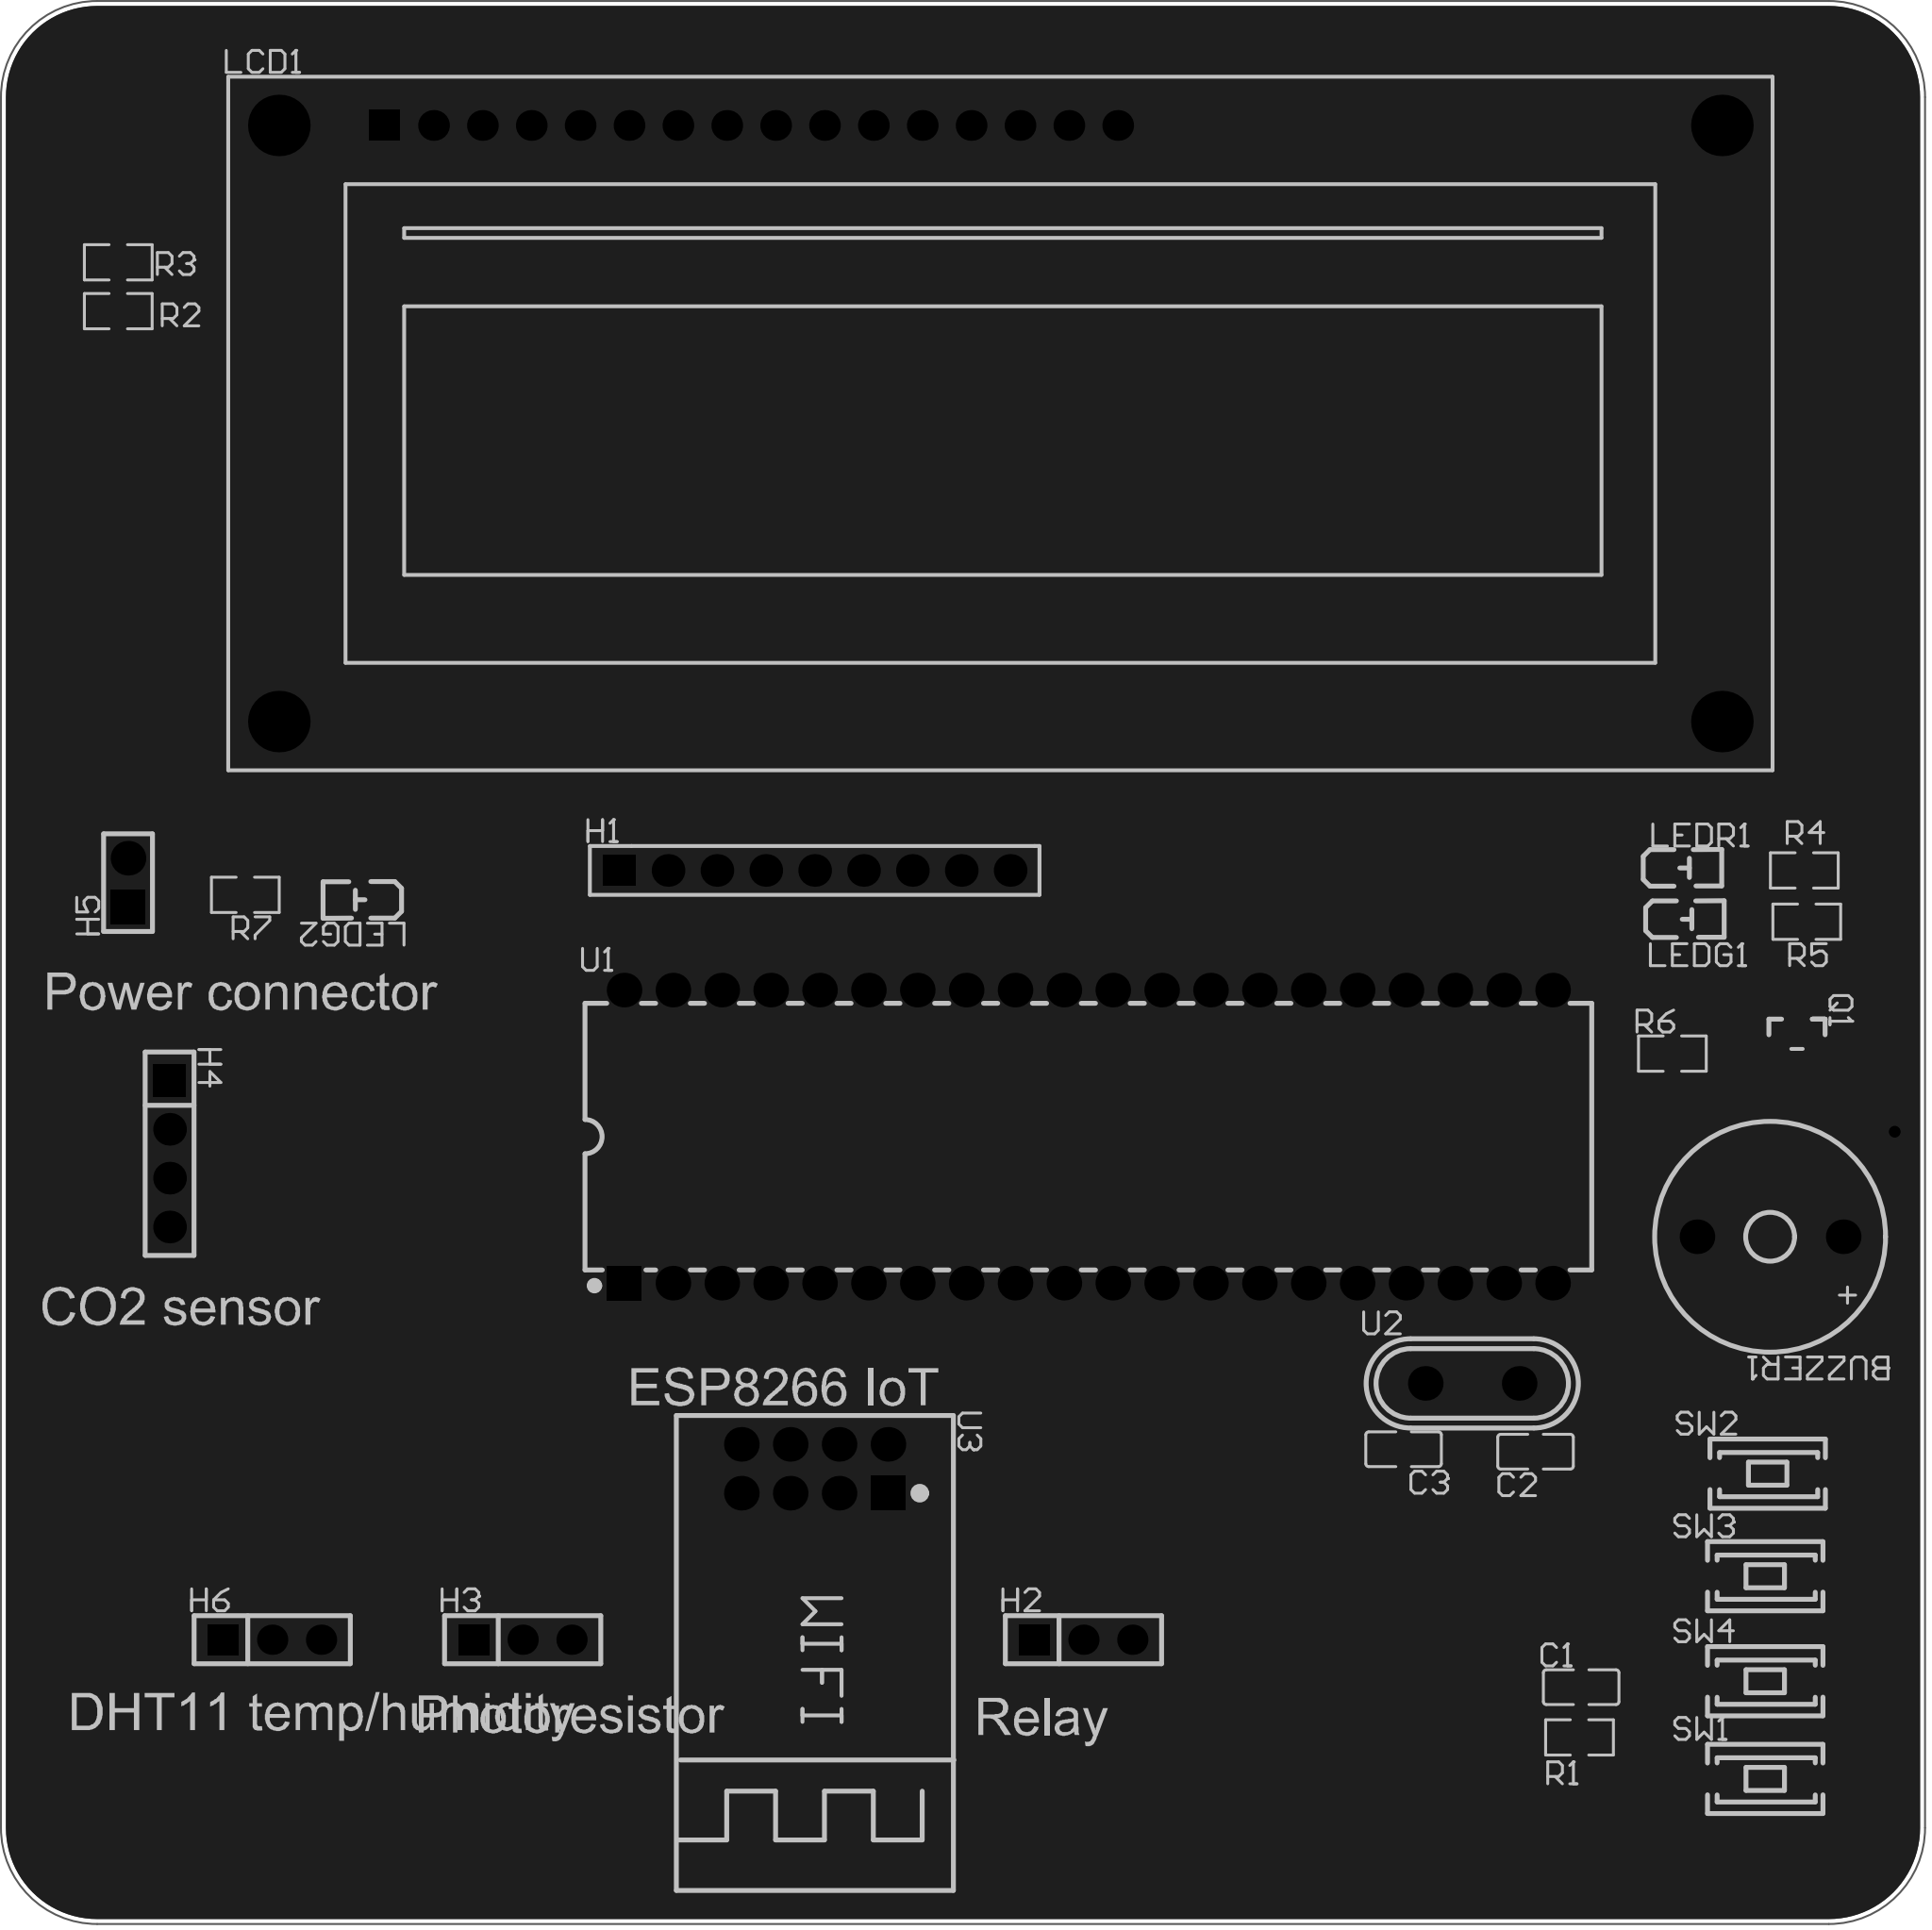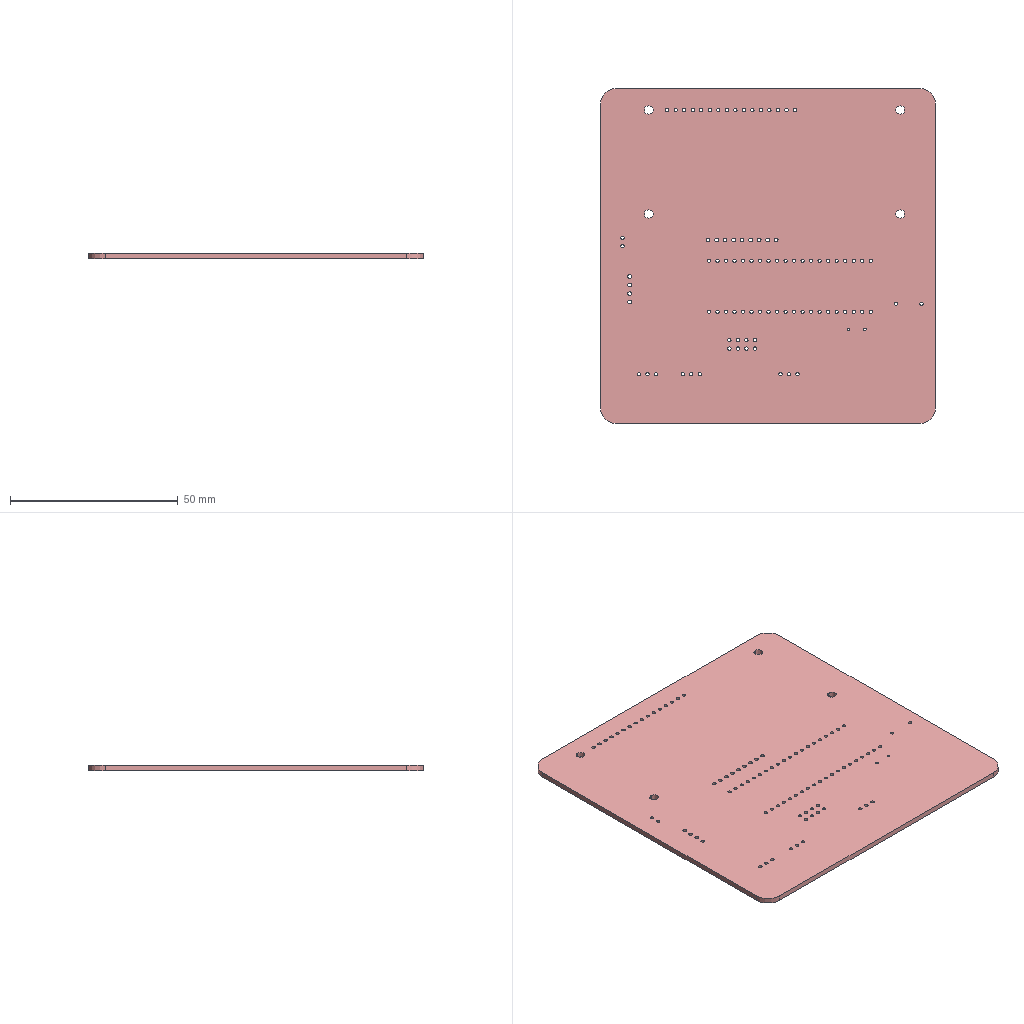Circuit board layout | Altium Designer | box 100 x 100 x 1.6 mm
Layer stack:
# Altium Designer layer stack of  (unit mm; dielectric type: 0 none, 1 core, 2 prepreg, 3 surface material)
index,name,kind,layer,copper_thickness_mm,dielectric_type,dielectric_thickness_mm,dielectric_material,dielectric_constant
0,Top Paste Mask Layer,other,,,,,,
1,Top Silkscreen Layer,other,,,,,,
2,Top Solder Mask Layer,dielectric,,,3,0.01,,3.3
3,Top Layer,copper,Top Layer,0.035,,,,
4,Dielectric1,dielectric,,,3,1.51,FR4,4.5
5,Bottom Layer,copper,Bottom Layer,0.035,,,,
6,Bottom Solder Mask Layer,dielectric,,,3,0.01,,3.3
7,Bottom Silkscreen Layer,other,,,,,,
8,Bottom Paste Mask Layer,other,,,,,,
# drill layer pairs: low layer,high layer
drill_pair,Top Layer,Bottom Layer
Part placement:
Designator,Comment,Layer,Footprint,Center-X(mm),Center-Y(mm),Rotation
BUZZER1,buzzer-12X9,TopLayer,BUZ-TH_BD12.0-P7.60-D0.6-FD,175.768,117.475,180
C1,10uf,TopLayer,C0805,165.947,94.052,0
C2,30pf,TopLayer,C0805,156.718,106.426,0
C3,30pf,TopLayer,C0805,163.576,106.299,180
H1,,TopLayer,HDR-TH_9P-P2.54-V-F-1,126.111,136.525,0
LCD1,LMB162ADC,TopLayer,LCD1602,135.763,159.766,0
LEDG1,,TopLayer,LED_0805,171.4,133.99,0
LEDR1,,TopLayer,LED_0805,171.273,136.657,0
Q1,2N3906S-RTK/PS,TopLayer,SOT-23-3_L2.9-W1.3-P1.90-LS2.4-TR,177.165,128.143,270
R1,10K,TopLayer,R0805,165.862,91.44,0
R2,10K,TopLayer,R0805,89.916,165.608,180
R3,1K,TopLayer,R0805,89.916,168.148,0
R4,220,TopLayer,R0805,177.546,136.525,0
R5,220,TopLayer,R0805,177.673,133.858,0
R6,2.2K,TopLayer,R0805,170.688,127,0
U1,STC89C516RD+40I-PDIP40,TopLayer,DIP-40_L52.3-W13.9-P2.54-LS15.2-BL,140.335,122.682,0
U2,11.059MHz,TopLayer,HC-49US_L11.0-W4.6-P4.88,160.287,109.85,0
LEDG2,,TopLayer,LED_0805,102.539,134.996,180
R7,220,TopLayer,R0805,96.52,135.255,180
H5,,TopLayer,HDR-TH_2P-P2.54-V-M-1,90.424,135.89,90
SW1,Tact switch 3*6*2.5,TopLayer,SW-SMD_L6.0-W3.6-LS8.0,175.514,89.281,0
SW2,Tact switch 3*6*2.5,TopLayer,SW-SMD_L6.0-W3.6-LS8.0,175.641,105.156,0
SW3,Tact switch 3*6*2.5,TopLayer,SW-SMD_L6.0-W3.6-LS8.0,175.514,99.822,0
SW4,Tact switch 3*6*2.5,TopLayer,SW-SMD_L6.0-W3.6-LS8.0,175.514,94.361,0
H2,,TopLayer,HDR-TH_3P-P2.54-V-F,140.081,96.52,0
H3,,TopLayer,HDR-TH_3P-P2.54-V-F,110.934,96.52,0
H4,,TopLayer,HDR-TH_4P-P2.54-V-F,92.583,121.793,270
H6,,TopLayer,HDR-TH_3P-P2.54-V-F,97.917,96.52,0
U3,Ai-Thinker ESP-01S ESP8266,TopLayer,WIFIM-TH_8P-L24.7-W14.4-P2.54,126.111,105.41,270
Pad and via stacks:
# Altium Designer via and pad stacks of  (unit mm). Each distinct definition once, with the count of objects using it.
# via: kind,start_layer,end_layer,hole_mm,diameter_mm,mode(0 simple;1 top-mid-bottom;2 full stack),diameter_per_layer,count,example_net
# pad: kind,layer,hole_mm,hole_type(0 round;1 square;2 slot),plating,top_size,top_shape(1 round;2 rect;3 octagon;9 rounded rect),mid_size,bottom_size,mode,footprint,size_per_layer,count,example
pad,Multi-Layer,1,0,plated,1.8x1.8,1,1.8x1.8,1.8x1.8,0,BUZ-TH_BD12.0-P7.60-D0.6-FD,,2,BUZZER1.2
pad,Multi-Layer,1.1,0,plated,1.7x1.575,2,1.7x1.575,1.7x1.575,0,HDR-TH_9P-P2.54-V-F-1,,1,H1.1
pad,Multi-Layer,1.1,0,plated,1.7x1.7,1,1.7x1.7,1.7x1.7,0,HDR-TH_9P-P2.54-V-F-1,,8,H1.2
pad,Multi-Layer,1,0,plated,1.6x1.6,1,1.6x1.6,1.6x1.6,0,LCD1602,,15,LCD1.16
pad,Multi-Layer,1,0,plated,1.6x1.6,2,1.6x1.6,1.6x1.6,0,LCD1602,,1,LCD1.1
pad,Multi-Layer,2.5,2,plated,3.2x3.2,1,3.2x3.2,3.2x3.2,0,LCD1602,,4,LCD1.0
pad,Multi-Layer,1,0,plated,1.8x1.8,1,1.8x1.8,1.8x1.8,0,DIP-40_L52.3-W13.9-P2.54-LS15.2-BL,,39,U1.19
pad,Multi-Layer,1,0,plated,1.8x1.8,2,1.8x1.8,1.8x1.8,0,DIP-40_L52.3-W13.9-P2.54-LS15.2-BL,,1,U1.1
pad,Multi-Layer,0.8,0,plated,1.8x1.8,1,1.8x1.8,1.8x1.8,0,HC-49US_L11.0-W4.6-P4.88,,2,U2.1
pad,Multi-Layer,1,0,plated,1.8x1.8,1,1.8x1.8,1.8x1.8,0,HDR-TH_2P-P2.54-V-M-1,,1,H5.2
pad,Multi-Layer,1,0,plated,1.8x1.8,2,1.8x1.8,1.8x1.8,0,HDR-TH_2P-P2.54-V-M-1,,1,H5.1
pad,Multi-Layer,1.02,0,plated,1.575x1.575,1,1.575x1.575,1.575x1.575,0,HDR-TH_3P-P2.54-V-F,,6,H2.3
pad,Multi-Layer,1.02,0,plated,1.575x1.575,2,1.575x1.575,1.575x1.575,0,HDR-TH_3P-P2.54-V-F,,3,H2.1
pad,Multi-Layer,1.1,0,plated,1.7x1.7,2,1.7x1.7,1.7x1.7,0,HDR-TH_4P-P2.54-V-F,,1,H4.1
pad,Multi-Layer,1.1,0,plated,1.7x1.7,1,1.7x1.7,1.7x1.7,0,HDR-TH_4P-P2.54-V-F,,3,H4.2
pad,Multi-Layer,1,0,plated,1.8x1.8,1,1.8x1.8,1.8x1.8,0,WIFIM-TH_8P-L24.7-W14.4-P2.54,,7,U3.8
pad,Multi-Layer,1,0,plated,1.8x1.8,2,1.8x1.8,1.8x1.8,0,WIFIM-TH_8P-L24.7-W14.4-P2.54,,1,U3.1
pad,Top Layer,0,0,plated,1.41x1.35,2,1.41x1.35,1.41x1.35,0,C0805,,6,C1.2
pad,Top Layer,0,0,plated,1x1.25,2,1x1.25,1x1.25,0,LED_0805,,6,LEDG1.2
pad,Top Layer,0,0,plated,0.7x1.25,2,0.7x1.25,0.7x1.25,0,SOT-23-3_L2.9-W1.3-P1.90-LS2.4-TR,,3,Q1.3
pad,Top Layer,0,0,plated,1.133x1.377,2,1.133x1.377,1.133x1.377,0,R0805,,14,R1.2
pad,Top Layer,0,0,plated,1.5x1,2,1.5x1,1.5x1,0,SW-SMD_L6.0-W3.6-LS8.0,,8,SW1.1
via,Top Layer,Bottom Layer,0.3048,0.61,0,,1,VCC
Copper pours:
name,layer,net,type(0 solid;1 hatched;2 none)
Top Layer-GND,Top Layer,GND,0
Bottom Layer-GND,Bottom Layer,GND,0